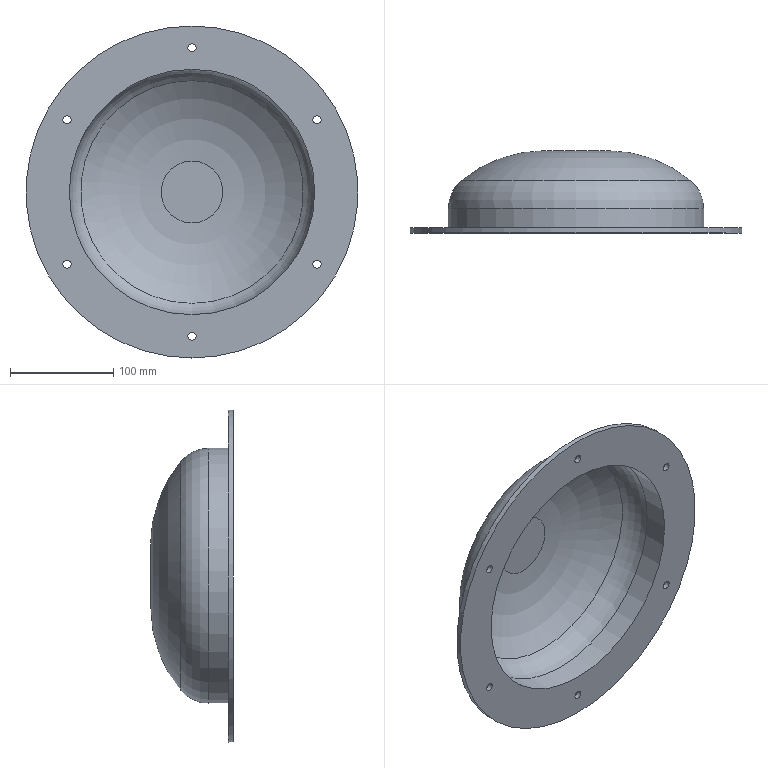Part | STEP file | JBJ-P-1000-05 | 1 solid | 17 faces | box 322 x 80 x 322 mm | volume 568917 mm3 | cylinder 9 | torus 4 | plane 4 | commonest cylinder face diameters 8 x6 238 x1 248 x1 322 x1
STEP:
#1=CARTESIAN_POINT('',(0.,822.534,119.));
#2=VERTEX_POINT('',#1);
#3=CARTESIAN_POINT('',(0.,822.534,-0.000000001));
#4=DIRECTION('',(0.,1.,0.));
#5=DIRECTION('',(0.,0.,1.));
#6=AXIS2_PLACEMENT_3D('',#3,#4,#5);
#7=CIRCLE('',#6,119.);
#8=EDGE_CURVE('',#2,#2,#7,.T.);
#9=ORIENTED_EDGE('',*,*,#8,.F.);
#10=EDGE_LOOP('',(#9));
#11=FACE_OUTER_BOUND('',#10,.T.);
#12=CARTESIAN_POINT('',(0.,845.689,108.074));
#13=VERTEX_POINT('',#12);
#14=CARTESIAN_POINT('',(0.,845.689,-0.000000001));
#15=DIRECTION('',(0.,1.,0.));
#16=DIRECTION('',(0.,0.,1.));
#17=AXIS2_PLACEMENT_3D('',#14,#15,#16);
#18=CIRCLE('',#17,108.074);
#19=EDGE_CURVE('',#13,#13,#18,.T.);
#20=ORIENTED_EDGE('',*,*,#19,.T.);
#21=EDGE_LOOP('',(#20));
#22=FACE_OUTER_BOUND('',#21,.T.);
#23=CARTESIAN_POINT('',(0.,822.534,-0.000000001));
#24=DIRECTION('',(0.,1.,0.));
#25=DIRECTION('',(0.,0.,1.));
#26=AXIS2_PLACEMENT_3D('',#23,#24,#25);
#27=TOROIDAL_SURFACE('',#26,89.,30.);
#28=ADVANCED_FACE('',(#11,#22),#27,.F.);
#29=ORIENTED_EDGE('',*,*,#19,.F.);
#30=EDGE_LOOP('',(#29));
#31=FACE_OUTER_BOUND('',#30,.T.);
#32=CARTESIAN_POINT('',(0.,873.705,29.998));
#33=VERTEX_POINT('',#32);
#34=CARTESIAN_POINT('',(0.,873.705,-0.000000001));
#35=DIRECTION('',(0.,1.,0.));
#36=DIRECTION('',(0.,0.,1.));
#37=AXIS2_PLACEMENT_3D('',#34,#35,#36);
#38=CIRCLE('',#37,29.998);
#39=EDGE_CURVE('',#33,#33,#38,.T.);
#40=ORIENTED_EDGE('',*,*,#39,.T.);
#41=EDGE_LOOP('',(#40));
#42=FACE_OUTER_BOUND('',#41,.T.);
#43=CARTESIAN_POINT('',(0.,750.905,0.));
#44=DIRECTION('',(0.,1.,0.));
#45=DIRECTION('',(0.,0.,1.));
#46=AXIS2_PLACEMENT_3D('',#43,#44,#45);
#47=TOROIDAL_SURFACE('',#46,29.998,122.8);
#48=ADVANCED_FACE('',(#31,#42),#47,.F.);
#49=ORIENTED_EDGE('',*,*,#39,.F.);
#50=EDGE_LOOP('',(#49));
#51=FACE_OUTER_BOUND('',#50,.T.);
#52=CARTESIAN_POINT('',(0.,873.705,0.));
#53=DIRECTION('',(0.,1.,0.));
#54=DIRECTION('',(0.,0.,1.));
#55=AXIS2_PLACEMENT_3D('',#52,#53,#54);
#56=PLANE('',#55);
#57=ADVANCED_FACE('',(#51),#56,.F.);
#58=CARTESIAN_POINT('',(0.,878.705,29.998));
#59=VERTEX_POINT('',#58);
#60=CARTESIAN_POINT('',(0.,878.705,-0.000000001));
#61=DIRECTION('',(0.,1.,0.));
#62=DIRECTION('',(0.,0.,1.));
#63=AXIS2_PLACEMENT_3D('',#60,#61,#62);
#64=CIRCLE('',#63,29.998);
#65=EDGE_CURVE('',#59,#59,#64,.T.);
#66=ORIENTED_EDGE('',*,*,#65,.T.);
#67=EDGE_LOOP('',(#66));
#68=FACE_OUTER_BOUND('',#67,.T.);
#69=CARTESIAN_POINT('',(0.,878.705,0.));
#70=DIRECTION('',(0.,1.,0.));
#71=DIRECTION('',(0.,0.,1.));
#72=AXIS2_PLACEMENT_3D('',#69,#70,#71);
#73=PLANE('',#72);
#74=ADVANCED_FACE('',(#68),#73,.T.);
#75=CARTESIAN_POINT('',(0.,849.548,111.253));
#76=VERTEX_POINT('',#75);
#77=CARTESIAN_POINT('',(0.,849.548,-0.000000001));
#78=DIRECTION('',(0.,1.,0.));
#79=DIRECTION('',(0.,0.,1.));
#80=AXIS2_PLACEMENT_3D('',#77,#78,#79);
#81=CIRCLE('',#80,111.253);
#82=EDGE_CURVE('',#76,#76,#81,.T.);
#83=ORIENTED_EDGE('',*,*,#82,.T.);
#84=EDGE_LOOP('',(#83));
#85=FACE_OUTER_BOUND('',#84,.T.);
#86=ORIENTED_EDGE('',*,*,#65,.F.);
#87=EDGE_LOOP('',(#86));
#88=FACE_OUTER_BOUND('',#87,.T.);
#89=CARTESIAN_POINT('',(0.,750.905,0.));
#90=DIRECTION('',(0.,1.,0.));
#91=DIRECTION('',(0.,0.,1.));
#92=AXIS2_PLACEMENT_3D('',#89,#90,#91);
#93=TOROIDAL_SURFACE('',#92,29.998,127.8);
#94=ADVANCED_FACE('',(#85,#88),#93,.T.);
#95=CARTESIAN_POINT('',(0.,822.534,124.));
#96=VERTEX_POINT('',#95);
#97=CARTESIAN_POINT('',(0.,822.534,-0.000000001));
#98=DIRECTION('',(0.,1.,0.));
#99=DIRECTION('',(0.,0.,1.));
#100=AXIS2_PLACEMENT_3D('',#97,#98,#99);
#101=CIRCLE('',#100,124.);
#102=EDGE_CURVE('',#96,#96,#101,.T.);
#103=ORIENTED_EDGE('',*,*,#102,.T.);
#104=EDGE_LOOP('',(#103));
#105=FACE_OUTER_BOUND('',#104,.T.);
#106=ORIENTED_EDGE('',*,*,#82,.F.);
#107=EDGE_LOOP('',(#106));
#108=FACE_OUTER_BOUND('',#107,.T.);
#109=CARTESIAN_POINT('',(0.,822.534,-0.000000001));
#110=DIRECTION('',(0.,1.,0.));
#111=DIRECTION('',(0.,0.,1.));
#112=AXIS2_PLACEMENT_3D('',#109,#110,#111);
#113=TOROIDAL_SURFACE('',#112,89.,35.);
#114=ADVANCED_FACE('',(#105,#108),#113,.T.);
#115=CARTESIAN_POINT('',(0.,803.705,124.));
#116=VERTEX_POINT('',#115);
#117=CARTESIAN_POINT('',(0.,803.705,-0.000000001));
#118=DIRECTION('',(0.,1.,0.));
#119=DIRECTION('',(0.,0.,1.));
#120=AXIS2_PLACEMENT_3D('',#117,#118,#119);
#121=CIRCLE('',#120,124.);
#122=EDGE_CURVE('',#116,#116,#121,.T.);
#123=ORIENTED_EDGE('',*,*,#122,.T.);
#124=EDGE_LOOP('',(#123));
#125=FACE_OUTER_BOUND('',#124,.T.);
#126=ORIENTED_EDGE('',*,*,#102,.F.);
#127=EDGE_LOOP('',(#126));
#128=FACE_OUTER_BOUND('',#127,.T.);
#129=CARTESIAN_POINT('',(0.,798.705,-0.000000001));
#130=DIRECTION('',(0.,1.,0.));
#131=DIRECTION('',(0.,0.,1.));
#132=AXIS2_PLACEMENT_3D('',#129,#130,#131);
#133=CYLINDRICAL_SURFACE('',#132,124.);
#134=ADVANCED_FACE('',(#125,#128),#133,.T.);
#135=CARTESIAN_POINT('',(0.,803.705,136.));
#136=VERTEX_POINT('',#135);
#137=CARTESIAN_POINT('',(0.,803.705,140.));
#138=DIRECTION('',(0.,-1.,0.));
#139=DIRECTION('',(0.,0.,-1.));
#140=AXIS2_PLACEMENT_3D('',#137,#138,#139);
#141=CIRCLE('',#140,4.);
#142=EDGE_CURVE('',#136,#136,#141,.T.);
#143=ORIENTED_EDGE('',*,*,#142,.T.);
#144=EDGE_LOOP('',(#143));
#145=FACE_BOUND('',#144,.T.);
#146=CARTESIAN_POINT('',(121.244,803.705,66.));
#147=VERTEX_POINT('',#146);
#148=CARTESIAN_POINT('',(121.244,803.705,70.));
#149=DIRECTION('',(0.,-1.,0.));
#150=DIRECTION('',(0.,0.,-1.));
#151=AXIS2_PLACEMENT_3D('',#148,#149,#150);
#152=CIRCLE('',#151,4.);
#153=EDGE_CURVE('',#147,#147,#152,.T.);
#154=ORIENTED_EDGE('',*,*,#153,.T.);
#155=EDGE_LOOP('',(#154));
#156=FACE_BOUND('',#155,.T.);
#157=CARTESIAN_POINT('',(121.244,803.705,-74.));
#158=VERTEX_POINT('',#157);
#159=CARTESIAN_POINT('',(121.244,803.705,-70.));
#160=DIRECTION('',(0.,-1.,0.));
#161=DIRECTION('',(0.,0.,-1.));
#162=AXIS2_PLACEMENT_3D('',#159,#160,#161);
#163=CIRCLE('',#162,4.);
#164=EDGE_CURVE('',#158,#158,#163,.T.);
#165=ORIENTED_EDGE('',*,*,#164,.T.);
#166=EDGE_LOOP('',(#165));
#167=FACE_BOUND('',#166,.T.);
#168=CARTESIAN_POINT('',(0.,803.705,-144.));
#169=VERTEX_POINT('',#168);
#170=CARTESIAN_POINT('',(0.,803.705,-140.));
#171=DIRECTION('',(0.,-1.,0.));
#172=DIRECTION('',(0.,0.,-1.));
#173=AXIS2_PLACEMENT_3D('',#170,#171,#172);
#174=CIRCLE('',#173,4.);
#175=EDGE_CURVE('',#169,#169,#174,.T.);
#176=ORIENTED_EDGE('',*,*,#175,.T.);
#177=EDGE_LOOP('',(#176));
#178=FACE_BOUND('',#177,.T.);
#179=CARTESIAN_POINT('',(-121.244,803.705,-74.));
#180=VERTEX_POINT('',#179);
#181=CARTESIAN_POINT('',(-121.244,803.705,-70.));
#182=DIRECTION('',(0.,-1.,0.));
#183=DIRECTION('',(0.,0.,-1.));
#184=AXIS2_PLACEMENT_3D('',#181,#182,#183);
#185=CIRCLE('',#184,4.);
#186=EDGE_CURVE('',#180,#180,#185,.T.);
#187=ORIENTED_EDGE('',*,*,#186,.T.);
#188=EDGE_LOOP('',(#187));
#189=FACE_BOUND('',#188,.T.);
#190=CARTESIAN_POINT('',(-121.244,803.705,66.));
#191=VERTEX_POINT('',#190);
#192=CARTESIAN_POINT('',(-121.244,803.705,70.));
#193=DIRECTION('',(0.,-1.,0.));
#194=DIRECTION('',(0.,0.,-1.));
#195=AXIS2_PLACEMENT_3D('',#192,#193,#194);
#196=CIRCLE('',#195,4.);
#197=EDGE_CURVE('',#191,#191,#196,.T.);
#198=ORIENTED_EDGE('',*,*,#197,.T.);
#199=EDGE_LOOP('',(#198));
#200=FACE_BOUND('',#199,.T.);
#201=ORIENTED_EDGE('',*,*,#122,.F.);
#202=EDGE_LOOP('',(#201));
#203=FACE_BOUND('',#202,.T.);
#204=CARTESIAN_POINT('',(0.,803.705,161.));
#205=VERTEX_POINT('',#204);
#206=CARTESIAN_POINT('',(0.,803.705,-0.000000001));
#207=DIRECTION('',(0.,1.,0.));
#208=DIRECTION('',(0.,0.,1.));
#209=AXIS2_PLACEMENT_3D('',#206,#207,#208);
#210=CIRCLE('',#209,161.);
#211=EDGE_CURVE('',#205,#205,#210,.T.);
#212=ORIENTED_EDGE('',*,*,#211,.T.);
#213=EDGE_LOOP('',(#212));
#214=FACE_OUTER_BOUND('',#213,.T.);
#215=CARTESIAN_POINT('',(0.,803.705,161.));
#216=DIRECTION('',(0.,-1.,0.));
#217=DIRECTION('',(0.,0.,-1.));
#218=AXIS2_PLACEMENT_3D('',#215,#216,#217);
#219=PLANE('',#218);
#220=ADVANCED_FACE('',(#145,#156,#167,#178,#189,#200,#203,#214),#219,.F.);
#221=ORIENTED_EDGE('',*,*,#211,.F.);
#222=EDGE_LOOP('',(#221));
#223=FACE_OUTER_BOUND('',#222,.T.);
#224=CARTESIAN_POINT('',(0.,798.705,161.));
#225=VERTEX_POINT('',#224);
#226=CARTESIAN_POINT('',(0.,798.705,-0.000000001));
#227=DIRECTION('',(0.,1.,0.));
#228=DIRECTION('',(0.,0.,1.));
#229=AXIS2_PLACEMENT_3D('',#226,#227,#228);
#230=CIRCLE('',#229,161.);
#231=EDGE_CURVE('',#225,#225,#230,.T.);
#232=ORIENTED_EDGE('',*,*,#231,.T.);
#233=EDGE_LOOP('',(#232));
#234=FACE_OUTER_BOUND('',#233,.T.);
#235=CARTESIAN_POINT('',(0.,798.705,-0.000000001));
#236=DIRECTION('',(0.,1.,0.));
#237=DIRECTION('',(0.,0.,1.));
#238=AXIS2_PLACEMENT_3D('',#235,#236,#237);
#239=CYLINDRICAL_SURFACE('',#238,161.);
#240=ADVANCED_FACE('',(#223,#234),#239,.T.);
#241=CARTESIAN_POINT('',(0.,798.705,136.));
#242=VERTEX_POINT('',#241);
#243=CARTESIAN_POINT('',(0.,798.705,140.));
#244=DIRECTION('',(0.,-1.,0.));
#245=DIRECTION('',(0.,0.,-1.));
#246=AXIS2_PLACEMENT_3D('',#243,#244,#245);
#247=CIRCLE('',#246,4.);
#248=EDGE_CURVE('',#242,#242,#247,.T.);
#249=ORIENTED_EDGE('',*,*,#248,.F.);
#250=EDGE_LOOP('',(#249));
#251=FACE_BOUND('',#250,.T.);
#252=CARTESIAN_POINT('',(121.244,798.705,66.));
#253=VERTEX_POINT('',#252);
#254=CARTESIAN_POINT('',(121.244,798.705,70.));
#255=DIRECTION('',(0.,-1.,0.));
#256=DIRECTION('',(0.,0.,-1.));
#257=AXIS2_PLACEMENT_3D('',#254,#255,#256);
#258=CIRCLE('',#257,4.);
#259=EDGE_CURVE('',#253,#253,#258,.T.);
#260=ORIENTED_EDGE('',*,*,#259,.F.);
#261=EDGE_LOOP('',(#260));
#262=FACE_BOUND('',#261,.T.);
#263=CARTESIAN_POINT('',(121.244,798.705,-74.));
#264=VERTEX_POINT('',#263);
#265=CARTESIAN_POINT('',(121.244,798.705,-70.));
#266=DIRECTION('',(0.,-1.,0.));
#267=DIRECTION('',(0.,0.,-1.));
#268=AXIS2_PLACEMENT_3D('',#265,#266,#267);
#269=CIRCLE('',#268,4.);
#270=EDGE_CURVE('',#264,#264,#269,.T.);
#271=ORIENTED_EDGE('',*,*,#270,.F.);
#272=EDGE_LOOP('',(#271));
#273=FACE_BOUND('',#272,.T.);
#274=CARTESIAN_POINT('',(0.,798.705,-144.));
#275=VERTEX_POINT('',#274);
#276=CARTESIAN_POINT('',(0.,798.705,-140.));
#277=DIRECTION('',(0.,-1.,0.));
#278=DIRECTION('',(0.,0.,-1.));
#279=AXIS2_PLACEMENT_3D('',#276,#277,#278);
#280=CIRCLE('',#279,4.);
#281=EDGE_CURVE('',#275,#275,#280,.T.);
#282=ORIENTED_EDGE('',*,*,#281,.F.);
#283=EDGE_LOOP('',(#282));
#284=FACE_BOUND('',#283,.T.);
#285=CARTESIAN_POINT('',(-121.244,798.705,-74.));
#286=VERTEX_POINT('',#285);
#287=CARTESIAN_POINT('',(-121.244,798.705,-70.));
#288=DIRECTION('',(0.,-1.,0.));
#289=DIRECTION('',(0.,0.,-1.));
#290=AXIS2_PLACEMENT_3D('',#287,#288,#289);
#291=CIRCLE('',#290,4.);
#292=EDGE_CURVE('',#286,#286,#291,.T.);
#293=ORIENTED_EDGE('',*,*,#292,.F.);
#294=EDGE_LOOP('',(#293));
#295=FACE_BOUND('',#294,.T.);
#296=CARTESIAN_POINT('',(-121.244,798.705,66.));
#297=VERTEX_POINT('',#296);
#298=CARTESIAN_POINT('',(-121.244,798.705,70.));
#299=DIRECTION('',(0.,-1.,0.));
#300=DIRECTION('',(0.,0.,-1.));
#301=AXIS2_PLACEMENT_3D('',#298,#299,#300);
#302=CIRCLE('',#301,4.);
#303=EDGE_CURVE('',#297,#297,#302,.T.);
#304=ORIENTED_EDGE('',*,*,#303,.F.);
#305=EDGE_LOOP('',(#304));
#306=FACE_BOUND('',#305,.T.);
#307=ORIENTED_EDGE('',*,*,#231,.F.);
#308=EDGE_LOOP('',(#307));
#309=FACE_OUTER_BOUND('',#308,.T.);
#310=CARTESIAN_POINT('',(0.,798.705,119.));
#311=VERTEX_POINT('',#310);
#312=CARTESIAN_POINT('',(0.,798.705,-0.000000001));
#313=DIRECTION('',(0.,1.,0.));
#314=DIRECTION('',(0.,0.,1.));
#315=AXIS2_PLACEMENT_3D('',#312,#313,#314);
#316=CIRCLE('',#315,119.);
#317=EDGE_CURVE('',#311,#311,#316,.T.);
#318=ORIENTED_EDGE('',*,*,#317,.T.);
#319=EDGE_LOOP('',(#318));
#320=FACE_BOUND('',#319,.T.);
#321=CARTESIAN_POINT('',(0.,798.705,119.));
#322=DIRECTION('',(0.,1.,0.));
#323=DIRECTION('',(0.,0.,1.));
#324=AXIS2_PLACEMENT_3D('',#321,#322,#323);
#325=PLANE('',#324);
#326=ADVANCED_FACE('',(#251,#262,#273,#284,#295,#306,#309,#320),#325,.F.);
#327=ORIENTED_EDGE('',*,*,#317,.F.);
#328=EDGE_LOOP('',(#327));
#329=FACE_OUTER_BOUND('',#328,.T.);
#330=ORIENTED_EDGE('',*,*,#8,.T.);
#331=EDGE_LOOP('',(#330));
#332=FACE_OUTER_BOUND('',#331,.T.);
#333=CARTESIAN_POINT('',(0.,798.705,-0.000000001));
#334=DIRECTION('',(0.,1.,0.));
#335=DIRECTION('',(0.,0.,1.));
#336=AXIS2_PLACEMENT_3D('',#333,#334,#335);
#337=CYLINDRICAL_SURFACE('',#336,119.);
#338=ADVANCED_FACE('',(#329,#332),#337,.F.);
#339=ORIENTED_EDGE('',*,*,#303,.T.);
#340=EDGE_LOOP('',(#339));
#341=FACE_OUTER_BOUND('',#340,.T.);
#342=ORIENTED_EDGE('',*,*,#197,.F.);
#343=EDGE_LOOP('',(#342));
#344=FACE_OUTER_BOUND('',#343,.T.);
#345=CARTESIAN_POINT('',(-121.244,798.705,70.));
#346=DIRECTION('',(0.,-1.,0.));
#347=DIRECTION('',(0.,0.,-1.));
#348=AXIS2_PLACEMENT_3D('',#345,#346,#347);
#349=CYLINDRICAL_SURFACE('',#348,4.);
#350=ADVANCED_FACE('',(#341,#344),#349,.F.);
#351=ORIENTED_EDGE('',*,*,#292,.T.);
#352=EDGE_LOOP('',(#351));
#353=FACE_OUTER_BOUND('',#352,.T.);
#354=ORIENTED_EDGE('',*,*,#186,.F.);
#355=EDGE_LOOP('',(#354));
#356=FACE_OUTER_BOUND('',#355,.T.);
#357=CARTESIAN_POINT('',(-121.244,798.705,-70.));
#358=DIRECTION('',(0.,-1.,0.));
#359=DIRECTION('',(0.,0.,-1.));
#360=AXIS2_PLACEMENT_3D('',#357,#358,#359);
#361=CYLINDRICAL_SURFACE('',#360,4.);
#362=ADVANCED_FACE('',(#353,#356),#361,.F.);
#363=ORIENTED_EDGE('',*,*,#281,.T.);
#364=EDGE_LOOP('',(#363));
#365=FACE_OUTER_BOUND('',#364,.T.);
#366=ORIENTED_EDGE('',*,*,#175,.F.);
#367=EDGE_LOOP('',(#366));
#368=FACE_OUTER_BOUND('',#367,.T.);
#369=CARTESIAN_POINT('',(0.,798.705,-140.));
#370=DIRECTION('',(0.,-1.,0.));
#371=DIRECTION('',(0.,0.,-1.));
#372=AXIS2_PLACEMENT_3D('',#369,#370,#371);
#373=CYLINDRICAL_SURFACE('',#372,4.);
#374=ADVANCED_FACE('',(#365,#368),#373,.F.);
#375=ORIENTED_EDGE('',*,*,#270,.T.);
#376=EDGE_LOOP('',(#375));
#377=FACE_OUTER_BOUND('',#376,.T.);
#378=ORIENTED_EDGE('',*,*,#164,.F.);
#379=EDGE_LOOP('',(#378));
#380=FACE_OUTER_BOUND('',#379,.T.);
#381=CARTESIAN_POINT('',(121.244,798.705,-70.));
#382=DIRECTION('',(0.,-1.,0.));
#383=DIRECTION('',(0.,0.,-1.));
#384=AXIS2_PLACEMENT_3D('',#381,#382,#383);
#385=CYLINDRICAL_SURFACE('',#384,4.);
#386=ADVANCED_FACE('',(#377,#380),#385,.F.);
#387=ORIENTED_EDGE('',*,*,#259,.T.);
#388=EDGE_LOOP('',(#387));
#389=FACE_OUTER_BOUND('',#388,.T.);
#390=ORIENTED_EDGE('',*,*,#153,.F.);
#391=EDGE_LOOP('',(#390));
#392=FACE_OUTER_BOUND('',#391,.T.);
#393=CARTESIAN_POINT('',(121.244,798.705,70.));
#394=DIRECTION('',(0.,-1.,0.));
#395=DIRECTION('',(0.,0.,-1.));
#396=AXIS2_PLACEMENT_3D('',#393,#394,#395);
#397=CYLINDRICAL_SURFACE('',#396,4.);
#398=ADVANCED_FACE('',(#389,#392),#397,.F.);
#399=ORIENTED_EDGE('',*,*,#248,.T.);
#400=EDGE_LOOP('',(#399));
#401=FACE_OUTER_BOUND('',#400,.T.);
#402=ORIENTED_EDGE('',*,*,#142,.F.);
#403=EDGE_LOOP('',(#402));
#404=FACE_OUTER_BOUND('',#403,.T.);
#405=CARTESIAN_POINT('',(0.,798.705,140.));
#406=DIRECTION('',(0.,-1.,0.));
#407=DIRECTION('',(0.,0.,-1.));
#408=AXIS2_PLACEMENT_3D('',#405,#406,#407);
#409=CYLINDRICAL_SURFACE('',#408,4.);
#410=ADVANCED_FACE('',(#401,#404),#409,.F.);
#411=CLOSED_SHELL('',(#28,#48,#57,#74,#94,#114,#134,#220,#240,#326,#338,#350,#362,#374,#386,#398,#410));
#412=MANIFOLD_SOLID_BREP('',#411);
#413=CARTESIAN_POINT('',(0.,0.,0.));
#414=DIRECTION('',(0.,0.,1.));
#415=DIRECTION('',(1.,0.,0.));
#416=AXIS2_PLACEMENT_3D('',#413,#414,#415);
#417=(LENGTH_UNIT()NAMED_UNIT(*)SI_UNIT(.MILLI.,.METRE.));
#418=UNCERTAINTY_MEASURE_WITH_UNIT(LENGTH_MEASURE(0.00001),#417,'','');
#419=(NAMED_UNIT(*)PLANE_ANGLE_UNIT()SI_UNIT($,.RADIAN.));
#420=(NAMED_UNIT(*)SI_UNIT($,.STERADIAN.)SOLID_ANGLE_UNIT());
#421=(GEOMETRIC_REPRESENTATION_CONTEXT(3)GLOBAL_UNCERTAINTY_ASSIGNED_CONTEXT((#418))GLOBAL_UNIT_ASSIGNED_CONTEXT((#417,#419,#420))REPRESENTATION_CONTEXT('',''));
#422=ADVANCED_BREP_SHAPE_REPRESENTATION('',(#412,#416),#421);